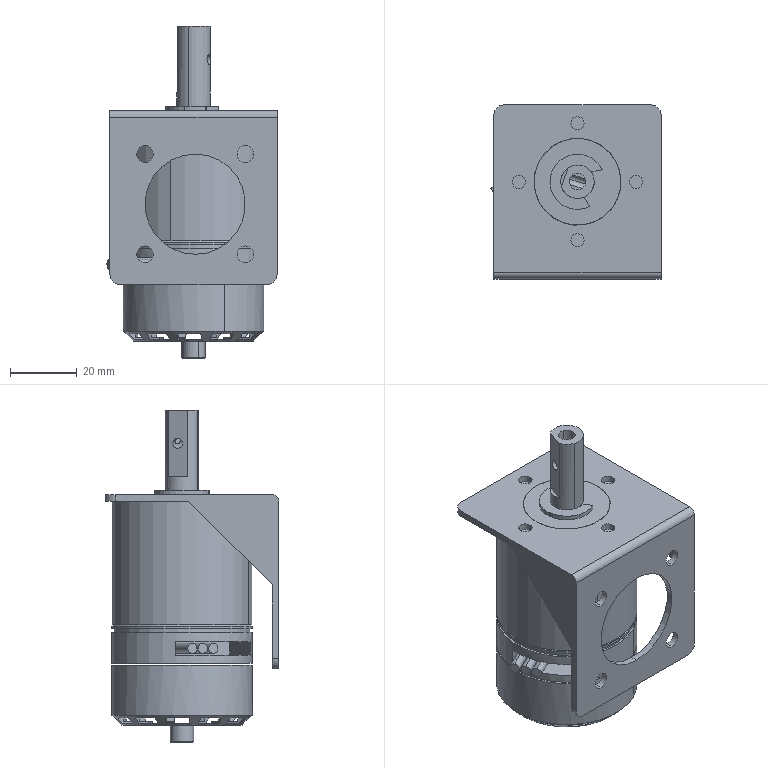Part | SolidWorks | 5 solids | 240 faces | box 50.9 x 52 x 99.3 mm | volume 84016 mm3 | plane 133 | cylinder 99 | cone 8 | commonest cylinder face diameters 4 x25 3 x20 5 x18 42 x8 10 x5 6 x4